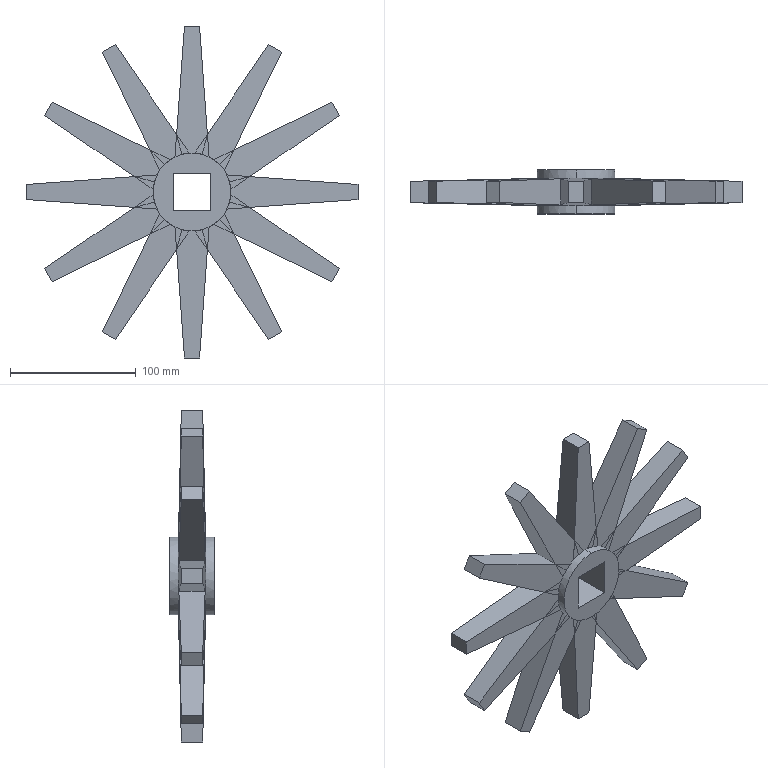Part | SolidWorks | features BaseBody 1 | 1 solid | 166 faces | box 264 x 35 x 264 mm | volume 515868 mm3 | plane 162 | cylinder 4 | commonest cylinder face diameters 62 x4